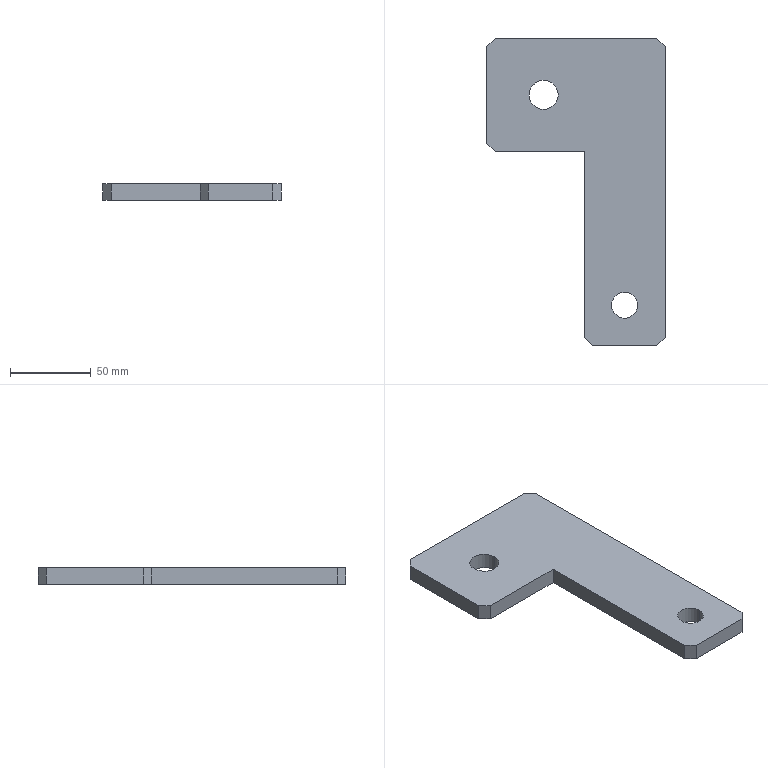Part | STEP file | POST.PLATE.3.stp | 1 solid | 17 faces | box 110 x 190 x 10 mm | volume 131820 mm3 | plane 9 | spline 6 | cylinder 2 | commonest cylinder face diameters 16 x2